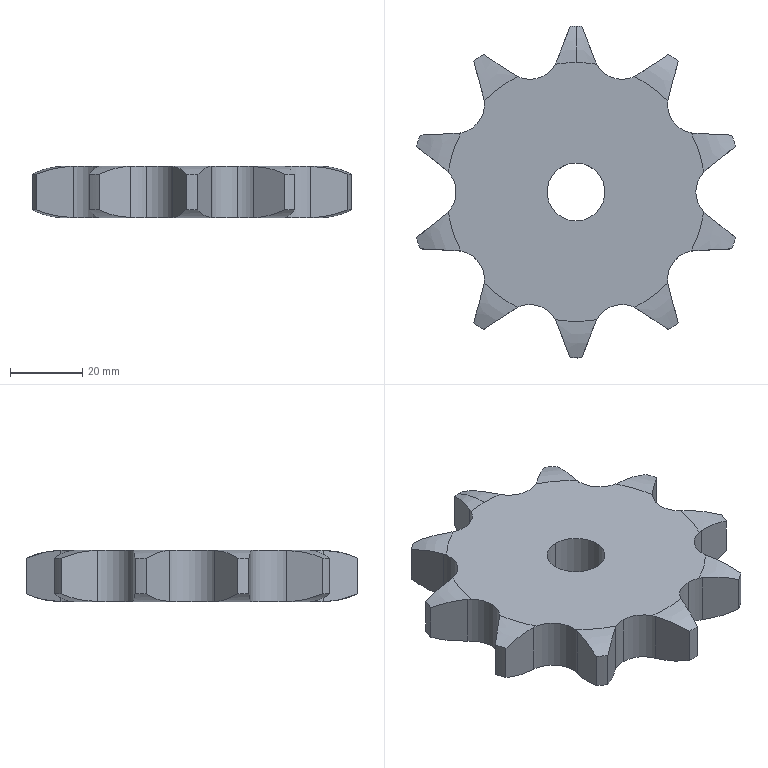Part | SolidWorks | features ICE 5, Revolution 5, CirPattern 3, LPattern 2 | 1 solid | 71 faces | box 88.261 x 91.8 x 14.2 mm | volume 61120 mm3 | cylinder 27 | torus 22 | plane 22 | commonest cylinder face diameters 15.88 x14 91.8 x11 16 x2